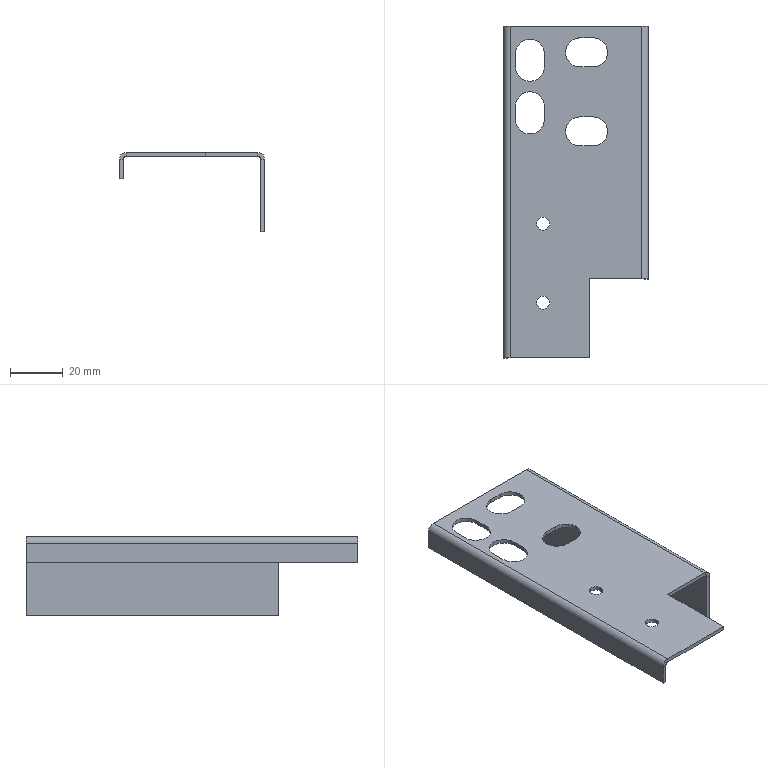Part | 1 solid | 46 faces | box 55 x 126 x 30 mm | volume 13884 mm3 | plane 28 | cylinder 18 | commonest cylinder face diameters 11 x10 5 x6 2 x2
STEP:
#1=CARTESIAN_POINT('',(12.,53.,-1.5));
#2=VERTEX_POINT('',#1);
#3=CARTESIAN_POINT('',(6.5,58.5,-1.5));
#4=VERTEX_POINT('',#3);
#5=CARTESIAN_POINT('',(6.5,53.,-1.5));
#6=DIRECTION('',(0.,0.,1.));
#7=DIRECTION('',(1.,0.,0.));
#8=AXIS2_PLACEMENT_3D('',#5,#6,#7);
#9=CIRCLE('',#8,5.5);
#10=EDGE_CURVE('',#2,#4,#9,.T.);
#11=ORIENTED_EDGE('',*,*,#10,.F.);
#12=CARTESIAN_POINT('',(12.,53.,0.));
#13=VERTEX_POINT('',#12);
#14=CARTESIAN_POINT('',(12.,53.,-10.));
#15=DIRECTION('',(0.,0.,1.));
#16=VECTOR('',#15,1000.);
#17=LINE('',#14,#16);
#18=EDGE_CURVE('',#2,#13,#17,.T.);
#19=ORIENTED_EDGE('',*,*,#18,.T.);
#20=CARTESIAN_POINT('',(6.5,58.5,0.));
#21=VERTEX_POINT('',#20);
#22=CARTESIAN_POINT('',(6.5,53.,0.));
#23=DIRECTION('',(0.,0.,1.));
#24=DIRECTION('',(1.,0.,0.));
#25=AXIS2_PLACEMENT_3D('',#22,#23,#24);
#26=CIRCLE('',#25,5.5);
#27=EDGE_CURVE('',#13,#21,#26,.T.);
#28=ORIENTED_EDGE('',*,*,#27,.T.);
#29=CARTESIAN_POINT('',(6.5,58.5,-10.));
#30=DIRECTION('',(0.,0.,1.));
#31=VECTOR('',#30,1000.);
#32=LINE('',#29,#31);
#33=EDGE_CURVE('',#4,#21,#32,.T.);
#34=ORIENTED_EDGE('',*,*,#33,.F.);
#35=EDGE_LOOP('',(#11,#19,#28,#34));
#36=FACE_OUTER_BOUND('',#35,.T.);
#37=CARTESIAN_POINT('',(6.5,53.,-10.));
#38=DIRECTION('',(0.,0.,1.));
#39=DIRECTION('',(1.,0.,0.));
#40=AXIS2_PLACEMENT_3D('',#37,#38,#39);
#41=CYLINDRICAL_SURFACE('',#40,5.5);
#42=ADVANCED_FACE('',(#36),#41,.F.);
#43=CARTESIAN_POINT('',(12.,23.,-1.5));
#44=VERTEX_POINT('',#43);
#45=CARTESIAN_POINT('',(6.5,28.5,-1.5));
#46=VERTEX_POINT('',#45);
#47=CARTESIAN_POINT('',(6.5,23.,-1.5));
#48=DIRECTION('',(0.,0.,1.));
#49=DIRECTION('',(1.,0.,0.));
#50=AXIS2_PLACEMENT_3D('',#47,#48,#49);
#51=CIRCLE('',#50,5.5);
#52=EDGE_CURVE('',#44,#46,#51,.T.);
#53=ORIENTED_EDGE('',*,*,#52,.F.);
#54=CARTESIAN_POINT('',(12.,23.,0.));
#55=VERTEX_POINT('',#54);
#56=CARTESIAN_POINT('',(12.,23.,-10.));
#57=DIRECTION('',(0.,0.,1.));
#58=VECTOR('',#57,1000.);
#59=LINE('',#56,#58);
#60=EDGE_CURVE('',#44,#55,#59,.T.);
#61=ORIENTED_EDGE('',*,*,#60,.T.);
#62=CARTESIAN_POINT('',(6.5,28.5,0.));
#63=VERTEX_POINT('',#62);
#64=CARTESIAN_POINT('',(6.5,23.,0.));
#65=DIRECTION('',(0.,0.,1.));
#66=DIRECTION('',(1.,0.,0.));
#67=AXIS2_PLACEMENT_3D('',#64,#65,#66);
#68=CIRCLE('',#67,5.5);
#69=EDGE_CURVE('',#55,#63,#68,.T.);
#70=ORIENTED_EDGE('',*,*,#69,.T.);
#71=CARTESIAN_POINT('',(6.5,28.5,-10.));
#72=DIRECTION('',(0.,0.,1.));
#73=VECTOR('',#72,1000.);
#74=LINE('',#71,#73);
#75=EDGE_CURVE('',#46,#63,#74,.T.);
#76=ORIENTED_EDGE('',*,*,#75,.F.);
#77=EDGE_LOOP('',(#53,#61,#70,#76));
#78=FACE_OUTER_BOUND('',#77,.T.);
#79=CARTESIAN_POINT('',(6.5,23.,-10.));
#80=DIRECTION('',(0.,0.,1.));
#81=DIRECTION('',(1.,0.,0.));
#82=AXIS2_PLACEMENT_3D('',#79,#80,#81);
#83=CYLINDRICAL_SURFACE('',#82,5.5);
#84=ADVANCED_FACE('',(#78),#83,.F.);
#85=CARTESIAN_POINT('',(-15.,-42.,-1.5));
#86=VERTEX_POINT('',#85);
#87=CARTESIAN_POINT('',(-10.,-42.,-1.5));
#88=VERTEX_POINT('',#87);
#89=CARTESIAN_POINT('',(-12.5,-42.,-1.5));
#90=DIRECTION('',(0.,0.,1.));
#91=DIRECTION('',(1.,0.,0.));
#92=AXIS2_PLACEMENT_3D('',#89,#90,#91);
#93=CIRCLE('',#92,2.5);
#94=EDGE_CURVE('',#86,#88,#93,.T.);
#95=ORIENTED_EDGE('',*,*,#94,.F.);
#96=CARTESIAN_POINT('',(-15.,-42.,0.));
#97=VERTEX_POINT('',#96);
#98=CARTESIAN_POINT('',(-15.,-42.,-10.));
#99=DIRECTION('',(0.,0.,1.));
#100=VECTOR('',#99,1000.);
#101=LINE('',#98,#100);
#102=EDGE_CURVE('',#86,#97,#101,.T.);
#103=ORIENTED_EDGE('',*,*,#102,.T.);
#104=CARTESIAN_POINT('',(-10.,-42.,0.));
#105=VERTEX_POINT('',#104);
#106=CARTESIAN_POINT('',(-12.5,-42.,0.));
#107=DIRECTION('',(0.,0.,1.));
#108=DIRECTION('',(1.,0.,0.));
#109=AXIS2_PLACEMENT_3D('',#106,#107,#108);
#110=CIRCLE('',#109,2.5);
#111=EDGE_CURVE('',#97,#105,#110,.T.);
#112=ORIENTED_EDGE('',*,*,#111,.T.);
#113=CARTESIAN_POINT('',(-10.,-42.,-10.));
#114=DIRECTION('',(0.,0.,1.));
#115=VECTOR('',#114,1000.);
#116=LINE('',#113,#115);
#117=EDGE_CURVE('',#88,#105,#116,.T.);
#118=ORIENTED_EDGE('',*,*,#117,.F.);
#119=EDGE_LOOP('',(#95,#103,#112,#118));
#120=FACE_OUTER_BOUND('',#119,.T.);
#121=CARTESIAN_POINT('',(-12.5,-42.,-10.));
#122=DIRECTION('',(0.,0.,1.));
#123=DIRECTION('',(1.,0.,0.));
#124=AXIS2_PLACEMENT_3D('',#121,#122,#123);
#125=CYLINDRICAL_SURFACE('',#124,2.5);
#126=ADVANCED_FACE('',(#120),#125,.F.);
#127=CARTESIAN_POINT('',(-15.,-12.,-1.5));
#128=VERTEX_POINT('',#127);
#129=CARTESIAN_POINT('',(-10.,-12.,-1.5));
#130=VERTEX_POINT('',#129);
#131=CARTESIAN_POINT('',(-12.5,-12.,-1.5));
#132=DIRECTION('',(0.,0.,1.));
#133=DIRECTION('',(1.,0.,0.));
#134=AXIS2_PLACEMENT_3D('',#131,#132,#133);
#135=CIRCLE('',#134,2.5);
#136=EDGE_CURVE('',#128,#130,#135,.T.);
#137=ORIENTED_EDGE('',*,*,#136,.F.);
#138=CARTESIAN_POINT('',(-15.,-12.,0.));
#139=VERTEX_POINT('',#138);
#140=CARTESIAN_POINT('',(-15.,-12.,-10.));
#141=DIRECTION('',(0.,0.,1.));
#142=VECTOR('',#141,1000.);
#143=LINE('',#140,#142);
#144=EDGE_CURVE('',#128,#139,#143,.T.);
#145=ORIENTED_EDGE('',*,*,#144,.T.);
#146=CARTESIAN_POINT('',(-10.,-12.,0.));
#147=VERTEX_POINT('',#146);
#148=CARTESIAN_POINT('',(-12.5,-12.,0.));
#149=DIRECTION('',(0.,0.,1.));
#150=DIRECTION('',(1.,0.,0.));
#151=AXIS2_PLACEMENT_3D('',#148,#149,#150);
#152=CIRCLE('',#151,2.5);
#153=EDGE_CURVE('',#139,#147,#152,.T.);
#154=ORIENTED_EDGE('',*,*,#153,.T.);
#155=CARTESIAN_POINT('',(-10.,-12.,-10.));
#156=DIRECTION('',(0.,0.,1.));
#157=VECTOR('',#156,1000.);
#158=LINE('',#155,#157);
#159=EDGE_CURVE('',#130,#147,#158,.T.);
#160=ORIENTED_EDGE('',*,*,#159,.F.);
#161=EDGE_LOOP('',(#137,#145,#154,#160));
#162=FACE_OUTER_BOUND('',#161,.T.);
#163=CARTESIAN_POINT('',(-12.5,-12.,-10.));
#164=DIRECTION('',(0.,0.,1.));
#165=DIRECTION('',(1.,0.,0.));
#166=AXIS2_PLACEMENT_3D('',#163,#164,#165);
#167=CYLINDRICAL_SURFACE('',#166,2.5);
#168=ADVANCED_FACE('',(#162),#167,.F.);
#169=CARTESIAN_POINT('',(27.5,-33.,-30.));
#170=VERTEX_POINT('',#169);
#171=CARTESIAN_POINT('',(27.5,-33.,-2.5));
#172=VERTEX_POINT('',#171);
#173=CARTESIAN_POINT('',(27.5,-33.,-30.));
#174=DIRECTION('',(0.,0.,1.));
#175=VECTOR('',#174,1000.);
#176=LINE('',#173,#175);
#177=EDGE_CURVE('',#170,#172,#176,.T.);
#178=ORIENTED_EDGE('',*,*,#177,.T.);
#179=CARTESIAN_POINT('',(26.,-33.,-2.5));
#180=VERTEX_POINT('',#179);
#181=CARTESIAN_POINT('',(27.5,-33.,-2.5));
#182=DIRECTION('',(-1.,0.,0.));
#183=VECTOR('',#182,1000.);
#184=LINE('',#181,#183);
#185=EDGE_CURVE('',#172,#180,#184,.T.);
#186=ORIENTED_EDGE('',*,*,#185,.T.);
#187=CARTESIAN_POINT('',(26.,-33.,-30.));
#188=VERTEX_POINT('',#187);
#189=CARTESIAN_POINT('',(26.,-33.,0.));
#190=DIRECTION('',(0.,0.,1.));
#191=VECTOR('',#190,1000.);
#192=LINE('',#189,#191);
#193=EDGE_CURVE('',#188,#180,#192,.T.);
#194=ORIENTED_EDGE('',*,*,#193,.F.);
#195=CARTESIAN_POINT('',(27.5,-33.,-30.));
#196=DIRECTION('',(-1.,0.,0.));
#197=VECTOR('',#196,1000.);
#198=LINE('',#195,#197);
#199=EDGE_CURVE('',#170,#188,#198,.T.);
#200=ORIENTED_EDGE('',*,*,#199,.F.);
#201=EDGE_LOOP('',(#178,#186,#194,#200));
#202=FACE_OUTER_BOUND('',#201,.T.);
#203=CARTESIAN_POINT('',(27.5,-33.,-30.));
#204=DIRECTION('',(0.,1.,0.));
#205=DIRECTION('',(0.,0.,1.));
#206=AXIS2_PLACEMENT_3D('',#203,#204,#205);
#207=PLANE('',#206);
#208=ADVANCED_FACE('',(#202),#207,.F.);
#209=CARTESIAN_POINT('',(25.,-33.,-1.5));
#210=VERTEX_POINT('',#209);
#211=CARTESIAN_POINT('',(5.,-33.,-1.5));
#212=VERTEX_POINT('',#211);
#213=CARTESIAN_POINT('',(0.,-33.,-1.5));
#214=DIRECTION('',(-1.,0.,0.));
#215=VECTOR('',#214,1000.);
#216=LINE('',#213,#215);
#217=EDGE_CURVE('',#210,#212,#216,.T.);
#218=ORIENTED_EDGE('',*,*,#217,.F.);
#219=CARTESIAN_POINT('',(25.,-33.,0.));
#220=VERTEX_POINT('',#219);
#221=CARTESIAN_POINT('',(25.,-33.,-1.5));
#222=DIRECTION('',(0.,0.,1.));
#223=VECTOR('',#222,1000.);
#224=LINE('',#221,#223);
#225=EDGE_CURVE('',#210,#220,#224,.T.);
#226=ORIENTED_EDGE('',*,*,#225,.T.);
#227=CARTESIAN_POINT('',(5.,-33.,0.));
#228=VERTEX_POINT('',#227);
#229=CARTESIAN_POINT('',(0.,-33.,0.));
#230=DIRECTION('',(-1.,0.,0.));
#231=VECTOR('',#230,1000.);
#232=LINE('',#229,#231);
#233=EDGE_CURVE('',#220,#228,#232,.T.);
#234=ORIENTED_EDGE('',*,*,#233,.T.);
#235=CARTESIAN_POINT('',(5.,-33.,-30.));
#236=DIRECTION('',(0.,0.,1.));
#237=VECTOR('',#236,1000.);
#238=LINE('',#235,#237);
#239=EDGE_CURVE('',#212,#228,#238,.T.);
#240=ORIENTED_EDGE('',*,*,#239,.F.);
#241=EDGE_LOOP('',(#218,#226,#234,#240));
#242=FACE_OUTER_BOUND('',#241,.T.);
#243=CARTESIAN_POINT('',(27.5,-33.,-30.));
#244=DIRECTION('',(0.,1.,0.));
#245=DIRECTION('',(0.,0.,1.));
#246=AXIS2_PLACEMENT_3D('',#243,#244,#245);
#247=PLANE('',#246);
#248=ADVANCED_FACE('',(#242),#247,.F.);
#249=CARTESIAN_POINT('',(-12.,47.5,-1.5));
#250=VERTEX_POINT('',#249);
#251=CARTESIAN_POINT('',(-12.,52.5,-1.5));
#252=VERTEX_POINT('',#251);
#253=CARTESIAN_POINT('',(-12.,0.,-1.5));
#254=DIRECTION('',(0.,1.,0.));
#255=VECTOR('',#254,1000.);
#256=LINE('',#253,#255);
#257=EDGE_CURVE('',#250,#252,#256,.T.);
#258=ORIENTED_EDGE('',*,*,#257,.T.);
#259=CARTESIAN_POINT('',(-23.,52.5,-1.5));
#260=VERTEX_POINT('',#259);
#261=CARTESIAN_POINT('',(-17.5,52.5,-1.5));
#262=DIRECTION('',(0.,0.,1.));
#263=DIRECTION('',(1.,0.,0.));
#264=AXIS2_PLACEMENT_3D('',#261,#262,#263);
#265=CIRCLE('',#264,5.5);
#266=EDGE_CURVE('',#252,#260,#265,.T.);
#267=ORIENTED_EDGE('',*,*,#266,.T.);
#268=CARTESIAN_POINT('',(-23.,47.5,-1.5));
#269=VERTEX_POINT('',#268);
#270=CARTESIAN_POINT('',(-23.,0.,-1.5));
#271=DIRECTION('',(0.,-1.,0.));
#272=VECTOR('',#271,1000.);
#273=LINE('',#270,#272);
#274=EDGE_CURVE('',#260,#269,#273,.T.);
#275=ORIENTED_EDGE('',*,*,#274,.T.);
#276=CARTESIAN_POINT('',(-17.5,47.5,-1.5));
#277=DIRECTION('',(0.,0.,1.));
#278=DIRECTION('',(1.,0.,0.));
#279=AXIS2_PLACEMENT_3D('',#276,#277,#278);
#280=CIRCLE('',#279,5.5);
#281=EDGE_CURVE('',#269,#250,#280,.T.);
#282=ORIENTED_EDGE('',*,*,#281,.T.);
#283=EDGE_LOOP('',(#258,#267,#275,#282));
#284=FACE_BOUND('',#283,.T.);
#285=CARTESIAN_POINT('',(-12.,27.5,-1.5));
#286=VERTEX_POINT('',#285);
#287=CARTESIAN_POINT('',(-12.,32.5,-1.5));
#288=VERTEX_POINT('',#287);
#289=CARTESIAN_POINT('',(-12.,0.,-1.5));
#290=DIRECTION('',(0.,1.,0.));
#291=VECTOR('',#290,1000.);
#292=LINE('',#289,#291);
#293=EDGE_CURVE('',#286,#288,#292,.T.);
#294=ORIENTED_EDGE('',*,*,#293,.T.);
#295=CARTESIAN_POINT('',(-23.,32.5,-1.5));
#296=VERTEX_POINT('',#295);
#297=CARTESIAN_POINT('',(-17.5,32.5,-1.5));
#298=DIRECTION('',(0.,0.,1.));
#299=DIRECTION('',(1.,0.,0.));
#300=AXIS2_PLACEMENT_3D('',#297,#298,#299);
#301=CIRCLE('',#300,5.5);
#302=EDGE_CURVE('',#288,#296,#301,.T.);
#303=ORIENTED_EDGE('',*,*,#302,.T.);
#304=CARTESIAN_POINT('',(-23.,27.5,-1.5));
#305=VERTEX_POINT('',#304);
#306=CARTESIAN_POINT('',(-23.,0.,-1.5));
#307=DIRECTION('',(0.,-1.,0.));
#308=VECTOR('',#307,1000.);
#309=LINE('',#306,#308);
#310=EDGE_CURVE('',#296,#305,#309,.T.);
#311=ORIENTED_EDGE('',*,*,#310,.T.);
#312=CARTESIAN_POINT('',(-17.5,27.5,-1.5));
#313=DIRECTION('',(0.,0.,1.));
#314=DIRECTION('',(1.,0.,0.));
#315=AXIS2_PLACEMENT_3D('',#312,#313,#314);
#316=CIRCLE('',#315,5.5);
#317=EDGE_CURVE('',#305,#286,#316,.T.);
#318=ORIENTED_EDGE('',*,*,#317,.T.);
#319=EDGE_LOOP('',(#294,#303,#311,#318));
#320=FACE_BOUND('',#319,.T.);
#321=CARTESIAN_POINT('',(1.5,58.5,-1.5));
#322=VERTEX_POINT('',#321);
#323=CARTESIAN_POINT('',(0.,58.5,-1.5));
#324=DIRECTION('',(-1.,0.,0.));
#325=VECTOR('',#324,1000.);
#326=LINE('',#323,#325);
#327=EDGE_CURVE('',#4,#322,#326,.T.);
#328=ORIENTED_EDGE('',*,*,#327,.T.);
#329=CARTESIAN_POINT('',(1.5,47.5,-1.5));
#330=VERTEX_POINT('',#329);
#331=CARTESIAN_POINT('',(1.5,53.,-1.5));
#332=DIRECTION('',(0.,0.,1.));
#333=DIRECTION('',(1.,0.,0.));
#334=AXIS2_PLACEMENT_3D('',#331,#332,#333);
#335=CIRCLE('',#334,5.5);
#336=EDGE_CURVE('',#322,#330,#335,.T.);
#337=ORIENTED_EDGE('',*,*,#336,.T.);
#338=CARTESIAN_POINT('',(6.5,47.5,-1.5));
#339=VERTEX_POINT('',#338);
#340=CARTESIAN_POINT('',(0.,47.5,-1.5));
#341=DIRECTION('',(1.,0.,0.));
#342=VECTOR('',#341,1000.);
#343=LINE('',#340,#342);
#344=EDGE_CURVE('',#330,#339,#343,.T.);
#345=ORIENTED_EDGE('',*,*,#344,.T.);
#346=CARTESIAN_POINT('',(6.5,53.,-1.5));
#347=DIRECTION('',(0.,0.,1.));
#348=DIRECTION('',(1.,0.,0.));
#349=AXIS2_PLACEMENT_3D('',#346,#347,#348);
#350=CIRCLE('',#349,5.5);
#351=EDGE_CURVE('',#339,#2,#350,.T.);
#352=ORIENTED_EDGE('',*,*,#351,.T.);
#353=ORIENTED_EDGE('',*,*,#10,.T.);
#354=EDGE_LOOP('',(#328,#337,#345,#352,#353));
#355=FACE_BOUND('',#354,.T.);
#356=CARTESIAN_POINT('',(1.5,28.5,-1.5));
#357=VERTEX_POINT('',#356);
#358=CARTESIAN_POINT('',(0.,28.5,-1.5));
#359=DIRECTION('',(-1.,0.,0.));
#360=VECTOR('',#359,1000.);
#361=LINE('',#358,#360);
#362=EDGE_CURVE('',#46,#357,#361,.T.);
#363=ORIENTED_EDGE('',*,*,#362,.T.);
#364=CARTESIAN_POINT('',(1.5,17.5,-1.5));
#365=VERTEX_POINT('',#364);
#366=CARTESIAN_POINT('',(1.5,23.,-1.5));
#367=DIRECTION('',(0.,0.,1.));
#368=DIRECTION('',(1.,0.,0.));
#369=AXIS2_PLACEMENT_3D('',#366,#367,#368);
#370=CIRCLE('',#369,5.5);
#371=EDGE_CURVE('',#357,#365,#370,.T.);
#372=ORIENTED_EDGE('',*,*,#371,.T.);
#373=CARTESIAN_POINT('',(6.5,17.5,-1.5));
#374=VERTEX_POINT('',#373);
#375=CARTESIAN_POINT('',(0.,17.5,-1.5));
#376=DIRECTION('',(1.,0.,0.));
#377=VECTOR('',#376,1000.);
#378=LINE('',#375,#377);
#379=EDGE_CURVE('',#365,#374,#378,.T.);
#380=ORIENTED_EDGE('',*,*,#379,.T.);
#381=CARTESIAN_POINT('',(6.5,23.,-1.5));
#382=DIRECTION('',(0.,0.,1.));
#383=DIRECTION('',(1.,0.,0.));
#384=AXIS2_PLACEMENT_3D('',#381,#382,#383);
#385=CIRCLE('',#384,5.5);
#386=EDGE_CURVE('',#374,#44,#385,.T.);
#387=ORIENTED_EDGE('',*,*,#386,.T.);
#388=ORIENTED_EDGE('',*,*,#52,.T.);
#389=EDGE_LOOP('',(#363,#372,#380,#387,#388));
#390=FACE_BOUND('',#389,.T.);
#391=CARTESIAN_POINT('',(-12.5,-42.,-1.5));
#392=DIRECTION('',(0.,0.,1.));
#393=DIRECTION('',(1.,0.,0.));
#394=AXIS2_PLACEMENT_3D('',#391,#392,#393);
#395=CIRCLE('',#394,2.5);
#396=EDGE_CURVE('',#88,#86,#395,.T.);
#397=ORIENTED_EDGE('',*,*,#396,.T.);
#398=ORIENTED_EDGE('',*,*,#94,.T.);
#399=EDGE_LOOP('',(#397,#398));
#400=FACE_BOUND('',#399,.T.);
#401=CARTESIAN_POINT('',(-12.5,-12.,-1.5));
#402=DIRECTION('',(0.,0.,1.));
#403=DIRECTION('',(1.,0.,0.));
#404=AXIS2_PLACEMENT_3D('',#401,#402,#403);
#405=CIRCLE('',#404,2.5);
#406=EDGE_CURVE('',#130,#128,#405,.T.);
#407=ORIENTED_EDGE('',*,*,#406,.T.);
#408=ORIENTED_EDGE('',*,*,#136,.T.);
#409=EDGE_LOOP('',(#407,#408));
#410=FACE_BOUND('',#409,.T.);
#411=ORIENTED_EDGE('',*,*,#217,.T.);
#412=CARTESIAN_POINT('',(5.,-63.,-1.5));
#413=VERTEX_POINT('',#412);
#414=CARTESIAN_POINT('',(5.,0.,-1.5));
#415=DIRECTION('',(0.,-1.,0.));
#416=VECTOR('',#415,1000.);
#417=LINE('',#414,#416);
#418=EDGE_CURVE('',#212,#413,#417,.T.);
#419=ORIENTED_EDGE('',*,*,#418,.T.);
#420=CARTESIAN_POINT('',(-25.,-63.,-1.5));
#421=VERTEX_POINT('',#420);
#422=CARTESIAN_POINT('',(-27.5,-63.,-1.5));
#423=DIRECTION('',(1.,0.,0.));
#424=VECTOR('',#423,1000.);
#425=LINE('',#422,#424);
#426=EDGE_CURVE('',#421,#413,#425,.T.);
#427=ORIENTED_EDGE('',*,*,#426,.F.);
#428=CARTESIAN_POINT('',(-25.,63.,-1.5));
#429=VERTEX_POINT('',#428);
#430=CARTESIAN_POINT('',(-25.,63.,-1.5));
#431=DIRECTION('',(0.,-1.,0.));
#432=VECTOR('',#431,1000.);
#433=LINE('',#430,#432);
#434=EDGE_CURVE('',#429,#421,#433,.T.);
#435=ORIENTED_EDGE('',*,*,#434,.F.);
#436=CARTESIAN_POINT('',(25.,63.,-1.5));
#437=VERTEX_POINT('',#436);
#438=CARTESIAN_POINT('',(-27.5,63.,-1.5));
#439=DIRECTION('',(-1.,0.,0.));
#440=VECTOR('',#439,1000.);
#441=LINE('',#438,#440);
#442=EDGE_CURVE('',#437,#429,#441,.T.);
#443=ORIENTED_EDGE('',*,*,#442,.F.);
#444=CARTESIAN_POINT('',(25.,-63.,-1.5));
#445=DIRECTION('',(0.,1.,0.));
#446=VECTOR('',#445,1000.);
#447=LINE('',#444,#446);
#448=EDGE_CURVE('',#210,#437,#447,.T.);
#449=ORIENTED_EDGE('',*,*,#448,.F.);
#450=EDGE_LOOP('',(#411,#419,#427,#435,#443,#449));
#451=FACE_OUTER_BOUND('',#450,.T.);
#452=CARTESIAN_POINT('',(0.,0.,-1.5));
#453=DIRECTION('',(0.,0.,1.));
#454=DIRECTION('',(1.,0.,0.));
#455=AXIS2_PLACEMENT_3D('',#452,#453,#454);
#456=PLANE('',#455);
#457=ADVANCED_FACE('',(#284,#320,#355,#390,#400,#410,#451),#456,.F.);
#458=CARTESIAN_POINT('',(-12.,52.5,0.));
#459=VERTEX_POINT('',#458);
#460=CARTESIAN_POINT('',(-23.,52.5,0.));
#461=VERTEX_POINT('',#460);
#462=CARTESIAN_POINT('',(-17.5,52.5,0.));
#463=DIRECTION('',(0.,0.,1.));
#464=DIRECTION('',(1.,0.,0.));
#465=AXIS2_PLACEMENT_3D('',#462,#463,#464);
#466=CIRCLE('',#465,5.5);
#467=EDGE_CURVE('',#459,#461,#466,.T.);
#468=ORIENTED_EDGE('',*,*,#467,.F.);
#469=CARTESIAN_POINT('',(-12.,47.5,0.));
#470=VERTEX_POINT('',#469);
#471=CARTESIAN_POINT('',(-12.,52.5,0.));
#472=DIRECTION('',(0.,1.,0.));
#473=VECTOR('',#472,1000.);
#474=LINE('',#471,#473);
#475=EDGE_CURVE('',#470,#459,#474,.T.);
#476=ORIENTED_EDGE('',*,*,#475,.F.);
#477=CARTESIAN_POINT('',(-23.,47.5,0.));
#478=VERTEX_POINT('',#477);
#479=CARTESIAN_POINT('',(-17.5,47.5,0.));
#480=DIRECTION('',(0.,0.,1.));
#481=DIRECTION('',(1.,0.,0.));
#482=AXIS2_PLACEMENT_3D('',#479,#480,#481);
#483=CIRCLE('',#482,5.5);
#484=EDGE_CURVE('',#478,#470,#483,.T.);
#485=ORIENTED_EDGE('',*,*,#484,.F.);
#486=CARTESIAN_POINT('',(-23.,52.5,0.));
#487=DIRECTION('',(0.,-1.,0.));
#488=VECTOR('',#487,1000.);
#489=LINE('',#486,#488);
#490=EDGE_CURVE('',#461,#478,#489,.T.);
#491=ORIENTED_EDGE('',*,*,#490,.F.);
#492=EDGE_LOOP('',(#468,#476,#485,#491));
#493=FACE_BOUND('',#492,.T.);
#494=CARTESIAN_POINT('',(-12.,32.5,0.));
#495=VERTEX_POINT('',#494);
#496=CARTESIAN_POINT('',(-23.,32.5,0.));
#497=VERTEX_POINT('',#496);
#498=CARTESIAN_POINT('',(-17.5,32.5,0.));
#499=DIRECTION('',(0.,0.,1.));
#500=DIRECTION('',(1.,0.,0.));
#501=AXIS2_PLACEMENT_3D('',#498,#499,#500);
#502=CIRCLE('',#501,5.5);
#503=EDGE_CURVE('',#495,#497,#502,.T.);
#504=ORIENTED_EDGE('',*,*,#503,.F.);
#505=CARTESIAN_POINT('',(-12.,27.5,0.));
#506=VERTEX_POINT('',#505);
#507=CARTESIAN_POINT('',(-12.,32.5,0.));
#508=DIRECTION('',(0.,1.,0.));
#509=VECTOR('',#508,1000.);
#510=LINE('',#507,#509);
#511=EDGE_CURVE('',#506,#495,#510,.T.);
#512=ORIENTED_EDGE('',*,*,#511,.F.);
#513=CARTESIAN_POINT('',(-23.,27.5,0.));
#514=VERTEX_POINT('',#513);
#515=CARTESIAN_POINT('',(-17.5,27.5,0.));
#516=DIRECTION('',(0.,0.,1.));
#517=DIRECTION('',(1.,0.,0.));
#518=AXIS2_PLACEMENT_3D('',#515,#516,#517);
#519=CIRCLE('',#518,5.5);
#520=EDGE_CURVE('',#514,#506,#519,.T.);
#521=ORIENTED_EDGE('',*,*,#520,.F.);
#522=CARTESIAN_POINT('',(-23.,32.5,0.));
#523=DIRECTION('',(0.,-1.,0.));
#524=VECTOR('',#523,1000.);
#525=LINE('',#522,#524);
#526=EDGE_CURVE('',#497,#514,#525,.T.);
#527=ORIENTED_EDGE('',*,*,#526,.F.);
#528=EDGE_LOOP('',(#504,#512,#521,#527));
#529=FACE_BOUND('',#528,.T.);
#530=CARTESIAN_POINT('',(1.5,58.5,0.));
#531=VERTEX_POINT('',#530);
#532=CARTESIAN_POINT('',(1.5,47.5,0.));
#533=VERTEX_POINT('',#532);
#534=CARTESIAN_POINT('',(1.5,53.,0.));
#535=DIRECTION('',(0.,0.,1.));
#536=DIRECTION('',(1.,0.,0.));
#537=AXIS2_PLACEMENT_3D('',#534,#535,#536);
#538=CIRCLE('',#537,5.5);
#539=EDGE_CURVE('',#531,#533,#538,.T.);
#540=ORIENTED_EDGE('',*,*,#539,.F.);
#541=CARTESIAN_POINT('',(1.5,58.5,0.));
#542=DIRECTION('',(-1.,0.,0.));
#543=VECTOR('',#542,1000.);
#544=LINE('',#541,#543);
#545=EDGE_CURVE('',#21,#531,#544,.T.);
#546=ORIENTED_EDGE('',*,*,#545,.F.);
#547=ORIENTED_EDGE('',*,*,#27,.F.);
#548=CARTESIAN_POINT('',(6.5,47.5,0.));
#549=VERTEX_POINT('',#548);
#550=CARTESIAN_POINT('',(6.5,53.,0.));
#551=DIRECTION('',(0.,0.,1.));
#552=DIRECTION('',(1.,0.,0.));
#553=AXIS2_PLACEMENT_3D('',#550,#551,#552);
#554=CIRCLE('',#553,5.5);
#555=EDGE_CURVE('',#549,#13,#554,.T.);
#556=ORIENTED_EDGE('',*,*,#555,.F.);
#557=CARTESIAN_POINT('',(1.5,47.5,0.));
#558=DIRECTION('',(1.,0.,0.));
#559=VECTOR('',#558,1000.);
#560=LINE('',#557,#559);
#561=EDGE_CURVE('',#533,#549,#560,.T.);
#562=ORIENTED_EDGE('',*,*,#561,.F.);
#563=EDGE_LOOP('',(#540,#546,#547,#556,#562));
#564=FACE_BOUND('',#563,.T.);
#565=CARTESIAN_POINT('',(1.5,28.5,0.));
#566=VERTEX_POINT('',#565);
#567=CARTESIAN_POINT('',(1.5,17.5,0.));
#568=VERTEX_POINT('',#567);
#569=CARTESIAN_POINT('',(1.5,23.,0.));
#570=DIRECTION('',(0.,0.,1.));
#571=DIRECTION('',(1.,0.,0.));
#572=AXIS2_PLACEMENT_3D('',#569,#570,#571);
#573=CIRCLE('',#572,5.5);
#574=EDGE_CURVE('',#566,#568,#573,.T.);
#575=ORIENTED_EDGE('',*,*,#574,.F.);
#576=CARTESIAN_POINT('',(1.5,28.5,0.));
#577=DIRECTION('',(-1.,0.,0.));
#578=VECTOR('',#577,1000.);
#579=LINE('',#576,#578);
#580=EDGE_CURVE('',#63,#566,#579,.T.);
#581=ORIENTED_EDGE('',*,*,#580,.F.);
#582=ORIENTED_EDGE('',*,*,#69,.F.);
#583=CARTESIAN_POINT('',(6.5,17.5,0.));
#584=VERTEX_POINT('',#583);
#585=CARTESIAN_POINT('',(6.5,23.,0.));
#586=DIRECTION('',(0.,0.,1.));
#587=DIRECTION('',(1.,0.,0.));
#588=AXIS2_PLACEMENT_3D('',#585,#586,#587);
#589=CIRCLE('',#588,5.5);
#590=EDGE_CURVE('',#584,#55,#589,.T.);
#591=ORIENTED_EDGE('',*,*,#590,.F.);
#592=CARTESIAN_POINT('',(1.5,17.5,0.));
#593=DIRECTION('',(1.,0.,0.));
#594=VECTOR('',#593,1000.);
#595=LINE('',#592,#594);
#596=EDGE_CURVE('',#568,#584,#595,.T.);
#597=ORIENTED_EDGE('',*,*,#596,.F.);
#598=EDGE_LOOP('',(#575,#581,#582,#591,#597));
#599=FACE_BOUND('',#598,.T.);
#600=CARTESIAN_POINT('',(-12.5,-42.,0.));
#601=DIRECTION('',(0.,0.,1.));
#602=DIRECTION('',(1.,0.,0.));
#603=AXIS2_PLACEMENT_3D('',#600,#601,#602);
#604=CIRCLE('',#603,2.5);
#605=EDGE_CURVE('',#105,#97,#604,.T.);
#606=ORIENTED_EDGE('',*,*,#605,.F.);
#607=ORIENTED_EDGE('',*,*,#111,.F.);
#608=EDGE_LOOP('',(#606,#607));
#609=FACE_BOUND('',#608,.T.);
#610=CARTESIAN_POINT('',(-12.5,-12.,0.));
#611=DIRECTION('',(0.,0.,1.));
#612=DIRECTION('',(1.,0.,0.));
#613=AXIS2_PLACEMENT_3D('',#610,#611,#612);
#614=CIRCLE('',#613,2.5);
#615=EDGE_CURVE('',#147,#139,#614,.T.);
#616=ORIENTED_EDGE('',*,*,#615,.F.);
#617=ORIENTED_EDGE('',*,*,#153,.F.);
#618=EDGE_LOOP('',(#616,#617));
#619=FACE_BOUND('',#618,.T.);
#620=CARTESIAN_POINT('',(5.,-63.,0.));
#621=VERTEX_POINT('',#620);
#622=CARTESIAN_POINT('',(5.,0.,0.));
#623=DIRECTION('',(0.,-1.,0.));
#624=VECTOR('',#623,1000.);
#625=LINE('',#622,#624);
#626=EDGE_CURVE('',#228,#621,#625,.T.);
#627=ORIENTED_EDGE('',*,*,#626,.F.);
#628=ORIENTED_EDGE('',*,*,#233,.F.);
#629=CARTESIAN_POINT('',(25.,63.,0.));
#630=VERTEX_POINT('',#629);
#631=CARTESIAN_POINT('',(25.,-63.,0.));
#632=DIRECTION('',(0.,1.,0.));
#633=VECTOR('',#632,1000.);
#634=LINE('',#631,#633);
#635=EDGE_CURVE('',#220,#630,#634,.T.);
#636=ORIENTED_EDGE('',*,*,#635,.T.);
#637=CARTESIAN_POINT('',(-25.,63.,0.));
#638=VERTEX_POINT('',#637);
#639=CARTESIAN_POINT('',(-27.5,63.,0.));
#640=DIRECTION('',(-1.,0.,0.));
#641=VECTOR('',#640,1000.);
#642=LINE('',#639,#641);
#643=EDGE_CURVE('',#630,#638,#642,.T.);
#644=ORIENTED_EDGE('',*,*,#643,.T.);
#645=CARTESIAN_POINT('',(-25.,-63.,0.));
#646=VERTEX_POINT('',#645);
#647=CARTESIAN_POINT('',(-25.,63.,0.));
#648=DIRECTION('',(0.,-1.,0.));
#649=VECTOR('',#648,1000.);
#650=LINE('',#647,#649);
#651=EDGE_CURVE('',#638,#646,#650,.T.);
#652=ORIENTED_EDGE('',*,*,#651,.T.);
#653=CARTESIAN_POINT('',(-27.5,-63.,0.));
#654=DIRECTION('',(1.,0.,0.));
#655=VECTOR('',#654,1000.);
#656=LINE('',#653,#655);
#657=EDGE_CURVE('',#646,#621,#656,.T.);
#658=ORIENTED_EDGE('',*,*,#657,.T.);
#659=EDGE_LOOP('',(#627,#628,#636,#644,#652,#658));
#660=FACE_OUTER_BOUND('',#659,.T.);
#661=CARTESIAN_POINT('',(0.,0.,0.));
#662=DIRECTION('',(0.,0.,1.));
#663=DIRECTION('',(1.,0.,0.));
#664=AXIS2_PLACEMENT_3D('',#661,#662,#663);
#665=PLANE('',#664);
#666=ADVANCED_FACE('',(#493,#529,#564,#599,#609,#619,#660),#665,.T.);
#667=ORIENTED_EDGE('',*,*,#442,.T.);
#668=CARTESIAN_POINT('',(-25.,63.,-1.5));
#669=DIRECTION('',(0.,0.,1.));
#670=VECTOR('',#669,1000.);
#671=LINE('',#668,#670);
#672=EDGE_CURVE('',#429,#638,#671,.T.);
#673=ORIENTED_EDGE('',*,*,#672,.T.);
#674=ORIENTED_EDGE('',*,*,#643,.F.);
#675=CARTESIAN_POINT('',(25.,63.,-1.5));
#676=DIRECTION('',(0.,0.,1.));
#677=VECTOR('',#676,1000.);
#678=LINE('',#675,#677);
#679=EDGE_CURVE('',#437,#630,#678,.T.);
#680=ORIENTED_EDGE('',*,*,#679,.F.);
#681=EDGE_LOOP('',(#667,#673,#674,#680));
#682=FACE_OUTER_BOUND('',#681,.T.);
#683=CARTESIAN_POINT('',(-27.5,63.,-1.5));
#684=DIRECTION('',(0.,1.,0.));
#685=DIRECTION('',(0.,0.,1.));
#686=AXIS2_PLACEMENT_3D('',#683,#684,#685);
#687=PLANE('',#686);
#688=ADVANCED_FACE('',(#682),#687,.T.);
#689=CARTESIAN_POINT('',(5.,-63.,-30.));
#690=DIRECTION('',(0.,0.,1.));
#691=VECTOR('',#690,1000.);
#692=LINE('',#689,#691);
#693=EDGE_CURVE('',#413,#621,#692,.T.);
#694=ORIENTED_EDGE('',*,*,#693,.T.);
#695=ORIENTED_EDGE('',*,*,#657,.F.);
#696=CARTESIAN_POINT('',(-25.,-63.,-1.5));
#697=DIRECTION('',(0.,0.,1.));
#698=VECTOR('',#697,1000.);
#699=LINE('',#696,#698);
#700=EDGE_CURVE('',#421,#646,#699,.T.);
#701=ORIENTED_EDGE('',*,*,#700,.F.);
#702=ORIENTED_EDGE('',*,*,#426,.T.);
#703=EDGE_LOOP('',(#694,#695,#701,#702));
#704=FACE_OUTER_BOUND('',#703,.T.);
#705=CARTESIAN_POINT('',(-27.5,-63.,-1.5));
#706=DIRECTION('',(0.,-1.,0.));
#707=DIRECTION('',(0.,0.,-1.));
#708=AXIS2_PLACEMENT_3D('',#705,#706,#707);
#709=PLANE('',#708);
#710=ADVANCED_FACE('',(#704),#709,.T.);
#711=CARTESIAN_POINT('',(26.,63.,-2.5));
#712=VERTEX_POINT('',#711);
#713=CARTESIAN_POINT('',(27.5,63.,-2.5));
#714=VERTEX_POINT('',#713);
#715=CARTESIAN_POINT('',(27.5,63.,-2.5));
#716=DIRECTION('',(1.,0.,0.));
#717=VECTOR('',#716,1000.);
#718=LINE('',#715,#717);
#719=EDGE_CURVE('',#712,#714,#718,.T.);
#720=ORIENTED_EDGE('',*,*,#719,.F.);
#721=CARTESIAN_POINT('',(25.,63.,-2.5));
#722=DIRECTION('',(0.,1.,0.));
#723=DIRECTION('',(0.,0.,-1.));
#724=AXIS2_PLACEMENT_3D('',#721,#722,#723);
#725=CIRCLE('',#724,1.);
#726=EDGE_CURVE('',#437,#712,#725,.T.);
#727=ORIENTED_EDGE('',*,*,#726,.F.);
#728=ORIENTED_EDGE('',*,*,#679,.T.);
#729=CARTESIAN_POINT('',(25.,63.,-2.5));
#730=DIRECTION('',(0.,1.,0.));
#731=DIRECTION('',(0.,0.,-1.));
#732=AXIS2_PLACEMENT_3D('',#729,#730,#731);
#733=CIRCLE('',#732,2.5);
#734=EDGE_CURVE('',#630,#714,#733,.T.);
#735=ORIENTED_EDGE('',*,*,#734,.T.);
#736=EDGE_LOOP('',(#720,#727,#728,#735));
#737=FACE_OUTER_BOUND('',#736,.T.);
#738=CARTESIAN_POINT('',(25.,63.,-2.5));
#739=DIRECTION('',(0.,1.,0.));
#740=DIRECTION('',(0.,0.,1.));
#741=AXIS2_PLACEMENT_3D('',#738,#739,#740);
#742=PLANE('',#741);
#743=ADVANCED_FACE('',(#737),#742,.T.);
#744=CARTESIAN_POINT('',(25.,-33.,-2.5));
#745=DIRECTION('',(0.,-1.,0.));
#746=DIRECTION('',(0.,0.,1.));
#747=AXIS2_PLACEMENT_3D('',#744,#745,#746);
#748=CIRCLE('',#747,2.5);
#749=EDGE_CURVE('',#172,#220,#748,.T.);
#750=ORIENTED_EDGE('',*,*,#749,.F.);
#751=CARTESIAN_POINT('',(27.5,0.,-2.5));
#752=DIRECTION('',(0.,-1.,0.));
#753=VECTOR('',#752,1000.);
#754=LINE('',#751,#753);
#755=EDGE_CURVE('',#714,#172,#754,.T.);
#756=ORIENTED_EDGE('',*,*,#755,.F.);
#757=ORIENTED_EDGE('',*,*,#734,.F.);
#758=ORIENTED_EDGE('',*,*,#635,.F.);
#759=EDGE_LOOP('',(#750,#756,#757,#758));
#760=FACE_OUTER_BOUND('',#759,.T.);
#761=CARTESIAN_POINT('',(25.,-63.,-2.5));
#762=DIRECTION('',(0.,-1.,0.));
#763=DIRECTION('',(1.,0.,0.));
#764=AXIS2_PLACEMENT_3D('',#761,#762,#763);
#765=CYLINDRICAL_SURFACE('',#764,2.5);
#766=ADVANCED_FACE('',(#760),#765,.T.);
#767=CARTESIAN_POINT('',(26.,63.,-2.5));
#768=DIRECTION('',(0.,-1.,0.));
#769=VECTOR('',#768,1000.);
#770=LINE('',#767,#769);
#771=EDGE_CURVE('',#712,#180,#770,.T.);
#772=ORIENTED_EDGE('',*,*,#771,.T.);
#773=CARTESIAN_POINT('',(25.,-33.,-2.5));
#774=DIRECTION('',(0.,-1.,0.));
#775=DIRECTION('',(0.,0.,1.));
#776=AXIS2_PLACEMENT_3D('',#773,#774,#775);
#777=CIRCLE('',#776,1.);
#778=EDGE_CURVE('',#180,#210,#777,.T.);
#779=ORIENTED_EDGE('',*,*,#778,.T.);
#780=ORIENTED_EDGE('',*,*,#448,.T.);
#781=ORIENTED_EDGE('',*,*,#726,.T.);
#782=EDGE_LOOP('',(#772,#779,#780,#781));
#783=FACE_OUTER_BOUND('',#782,.T.);
#784=CARTESIAN_POINT('',(25.,-63.,-2.5));
#785=DIRECTION('',(0.,-1.,0.));
#786=DIRECTION('',(1.,0.,0.));
#787=AXIS2_PLACEMENT_3D('',#784,#785,#786);
#788=CYLINDRICAL_SURFACE('',#787,1.);
#789=ADVANCED_FACE('',(#783),#788,.F.);
#790=CARTESIAN_POINT('',(26.,63.,-30.));
#791=VERTEX_POINT('',#790);
#792=CARTESIAN_POINT('',(26.,63.,0.));
#793=DIRECTION('',(0.,0.,-1.));
#794=VECTOR('',#793,1000.);
#795=LINE('',#792,#794);
#796=EDGE_CURVE('',#712,#791,#795,.T.);
#797=ORIENTED_EDGE('',*,*,#796,.F.);
#798=ORIENTED_EDGE('',*,*,#719,.T.);
#799=CARTESIAN_POINT('',(27.5,63.,-30.));
#800=VERTEX_POINT('',#799);
#801=CARTESIAN_POINT('',(27.5,63.,-30.));
#802=DIRECTION('',(0.,0.,-1.));
#803=VECTOR('',#802,1000.);
#804=LINE('',#801,#803);
#805=EDGE_CURVE('',#714,#800,#804,.T.);
#806=ORIENTED_EDGE('',*,*,#805,.T.);
#807=CARTESIAN_POINT('',(27.5,63.,-30.));
#808=DIRECTION('',(-1.,0.,0.));
#809=VECTOR('',#808,1000.);
#810=LINE('',#807,#809);
#811=EDGE_CURVE('',#800,#791,#810,.T.);
#812=ORIENTED_EDGE('',*,*,#811,.T.);
#813=EDGE_LOOP('',(#797,#798,#806,#812));
#814=FACE_OUTER_BOUND('',#813,.T.);
#815=CARTESIAN_POINT('',(27.5,63.,-30.));
#816=DIRECTION('',(0.,1.,0.));
#817=DIRECTION('',(-1.,0.,0.));
#818=AXIS2_PLACEMENT_3D('',#815,#816,#817);
#819=PLANE('',#818);
#820=ADVANCED_FACE('',(#814),#819,.T.);
#821=ORIENTED_EDGE('',*,*,#177,.F.);
#822=CARTESIAN_POINT('',(27.5,-63.,-30.));
#823=DIRECTION('',(0.,-1.,0.));
#824=VECTOR('',#823,1000.);
#825=LINE('',#822,#824);
#826=EDGE_CURVE('',#800,#170,#825,.T.);
#827=ORIENTED_EDGE('',*,*,#826,.F.);
#828=ORIENTED_EDGE('',*,*,#805,.F.);
#829=ORIENTED_EDGE('',*,*,#755,.T.);
#830=EDGE_LOOP('',(#821,#827,#828,#829));
#831=FACE_OUTER_BOUND('',#830,.T.);
#832=CARTESIAN_POINT('',(27.5,0.,0.));
#833=DIRECTION('',(1.,0.,0.));
#834=DIRECTION('',(0.,0.,-1.));
#835=AXIS2_PLACEMENT_3D('',#832,#833,#834);
#836=PLANE('',#835);
#837=ADVANCED_FACE('',(#831),#836,.T.);
#838=CARTESIAN_POINT('',(26.,0.,-30.));
#839=DIRECTION('',(0.,-1.,0.));
#840=VECTOR('',#839,1000.);
#841=LINE('',#838,#840);
#842=EDGE_CURVE('',#791,#188,#841,.T.);
#843=ORIENTED_EDGE('',*,*,#842,.T.);
#844=ORIENTED_EDGE('',*,*,#193,.T.);
#845=ORIENTED_EDGE('',*,*,#771,.F.);
#846=ORIENTED_EDGE('',*,*,#796,.T.);
#847=EDGE_LOOP('',(#843,#844,#845,#846));
#848=FACE_OUTER_BOUND('',#847,.T.);
#849=CARTESIAN_POINT('',(26.,0.,0.));
#850=DIRECTION('',(1.,0.,0.));
#851=DIRECTION('',(0.,0.,-1.));
#852=AXIS2_PLACEMENT_3D('',#849,#850,#851);
#853=PLANE('',#852);
#854=ADVANCED_FACE('',(#848),#853,.F.);
#855=ORIENTED_EDGE('',*,*,#199,.T.);
#856=ORIENTED_EDGE('',*,*,#842,.F.);
#857=ORIENTED_EDGE('',*,*,#811,.F.);
#858=ORIENTED_EDGE('',*,*,#826,.T.);
#859=EDGE_LOOP('',(#855,#856,#857,#858));
#860=FACE_OUTER_BOUND('',#859,.T.);
#861=CARTESIAN_POINT('',(27.5,-63.,-30.));
#862=DIRECTION('',(0.,0.,-1.));
#863=DIRECTION('',(-1.,0.,0.));
#864=AXIS2_PLACEMENT_3D('',#861,#862,#863);
#865=PLANE('',#864);
#866=ADVANCED_FACE('',(#860),#865,.T.);
#867=CARTESIAN_POINT('',(-26.,-63.,-2.5));
#868=VERTEX_POINT('',#867);
#869=CARTESIAN_POINT('',(-27.5,-63.,-2.5));
#870=VERTEX_POINT('',#869);
#871=CARTESIAN_POINT('',(-27.5,-63.,-2.5));
#872=DIRECTION('',(-1.,0.,0.));
#873=VECTOR('',#872,1000.);
#874=LINE('',#871,#873);
#875=EDGE_CURVE('',#868,#870,#874,.T.);
#876=ORIENTED_EDGE('',*,*,#875,.F.);
#877=CARTESIAN_POINT('',(-25.,-63.,-2.5));
#878=DIRECTION('',(0.,-1.,0.));
#879=DIRECTION('',(0.,0.,1.));
#880=AXIS2_PLACEMENT_3D('',#877,#878,#879);
#881=CIRCLE('',#880,1.);
#882=EDGE_CURVE('',#421,#868,#881,.T.);
#883=ORIENTED_EDGE('',*,*,#882,.F.);
#884=ORIENTED_EDGE('',*,*,#700,.T.);
#885=CARTESIAN_POINT('',(-25.,-63.,-2.5));
#886=DIRECTION('',(0.,-1.,0.));
#887=DIRECTION('',(0.,0.,1.));
#888=AXIS2_PLACEMENT_3D('',#885,#886,#887);
#889=CIRCLE('',#888,2.5);
#890=EDGE_CURVE('',#646,#870,#889,.T.);
#891=ORIENTED_EDGE('',*,*,#890,.T.);
#892=EDGE_LOOP('',(#876,#883,#884,#891));
#893=FACE_OUTER_BOUND('',#892,.T.);
#894=CARTESIAN_POINT('',(-25.,-63.,-2.5));
#895=DIRECTION('',(0.,-1.,0.));
#896=DIRECTION('',(0.,0.,-1.));
#897=AXIS2_PLACEMENT_3D('',#894,#895,#896);
#898=PLANE('',#897);
#899=ADVANCED_FACE('',(#893),#898,.T.);
#900=CARTESIAN_POINT('',(-26.,63.,-2.5));
#901=VERTEX_POINT('',#900);
#902=CARTESIAN_POINT('',(-25.,63.,-2.5));
#903=DIRECTION('',(0.,1.,0.));
#904=DIRECTION('',(0.,0.,1.));
#905=AXIS2_PLACEMENT_3D('',#902,#903,#904);
#906=CIRCLE('',#905,1.);
#907=EDGE_CURVE('',#901,#429,#906,.T.);
#908=ORIENTED_EDGE('',*,*,#907,.F.);
#909=CARTESIAN_POINT('',(-27.5,63.,-2.5));
#910=VERTEX_POINT('',#909);
#911=CARTESIAN_POINT('',(-26.,63.,-2.5));
#912=DIRECTION('',(-1.,0.,0.));
#913=VECTOR('',#912,1000.);
#914=LINE('',#911,#913);
#915=EDGE_CURVE('',#901,#910,#914,.T.);
#916=ORIENTED_EDGE('',*,*,#915,.T.);
#917=CARTESIAN_POINT('',(-25.,63.,-2.5));
#918=DIRECTION('',(0.,1.,0.));
#919=DIRECTION('',(0.,0.,1.));
#920=AXIS2_PLACEMENT_3D('',#917,#918,#919);
#921=CIRCLE('',#920,2.5);
#922=EDGE_CURVE('',#910,#638,#921,.T.);
#923=ORIENTED_EDGE('',*,*,#922,.T.);
#924=ORIENTED_EDGE('',*,*,#672,.F.);
#925=EDGE_LOOP('',(#908,#916,#923,#924));
#926=FACE_OUTER_BOUND('',#925,.T.);
#927=CARTESIAN_POINT('',(-25.,63.,-2.5));
#928=DIRECTION('',(0.,-1.,0.));
#929=DIRECTION('',(0.,0.,-1.));
#930=AXIS2_PLACEMENT_3D('',#927,#928,#929);
#931=PLANE('',#930);
#932=ADVANCED_FACE('',(#926),#931,.F.);
#933=ORIENTED_EDGE('',*,*,#651,.F.);
#934=ORIENTED_EDGE('',*,*,#922,.F.);
#935=CARTESIAN_POINT('',(-27.5,0.,-2.5));
#936=DIRECTION('',(0.,1.,0.));
#937=VECTOR('',#936,1000.);
#938=LINE('',#935,#937);
#939=EDGE_CURVE('',#870,#910,#938,.T.);
#940=ORIENTED_EDGE('',*,*,#939,.F.);
#941=ORIENTED_EDGE('',*,*,#890,.F.);
#942=EDGE_LOOP('',(#933,#934,#940,#941));
#943=FACE_OUTER_BOUND('',#942,.T.);
#944=CARTESIAN_POINT('',(-25.,63.,-2.5));
#945=DIRECTION('',(0.,1.,0.));
#946=DIRECTION('',(-1.,0.,0.));
#947=AXIS2_PLACEMENT_3D('',#944,#945,#946);
#948=CYLINDRICAL_SURFACE('',#947,2.5);
#949=ADVANCED_FACE('',(#943),#948,.T.);
#950=ORIENTED_EDGE('',*,*,#434,.T.);
#951=ORIENTED_EDGE('',*,*,#882,.T.);
#952=CARTESIAN_POINT('',(-26.,-63.,-2.5));
#953=DIRECTION('',(0.,1.,0.));
#954=VECTOR('',#953,1000.);
#955=LINE('',#952,#954);
#956=EDGE_CURVE('',#868,#901,#955,.T.);
#957=ORIENTED_EDGE('',*,*,#956,.T.);
#958=ORIENTED_EDGE('',*,*,#907,.T.);
#959=EDGE_LOOP('',(#950,#951,#957,#958));
#960=FACE_OUTER_BOUND('',#959,.T.);
#961=CARTESIAN_POINT('',(-25.,63.,-2.5));
#962=DIRECTION('',(0.,1.,0.));
#963=DIRECTION('',(-1.,0.,0.));
#964=AXIS2_PLACEMENT_3D('',#961,#962,#963);
#965=CYLINDRICAL_SURFACE('',#964,1.);
#966=ADVANCED_FACE('',(#960),#965,.F.);
#967=CARTESIAN_POINT('',(-27.5,63.,-10.));
#968=VERTEX_POINT('',#967);
#969=CARTESIAN_POINT('',(-27.5,63.,-1.5));
#970=DIRECTION('',(0.,0.,1.));
#971=VECTOR('',#970,1000.);
#972=LINE('',#969,#971);
#973=EDGE_CURVE('',#968,#910,#972,.T.);
#974=ORIENTED_EDGE('',*,*,#973,.T.);
#975=ORIENTED_EDGE('',*,*,#915,.F.);
#976=CARTESIAN_POINT('',(-26.,63.,-10.));
#977=VERTEX_POINT('',#976);
#978=CARTESIAN_POINT('',(-26.,63.,0.));
#979=DIRECTION('',(0.,0.,1.));
#980=VECTOR('',#979,1000.);
#981=LINE('',#978,#980);
#982=EDGE_CURVE('',#977,#901,#981,.T.);
#983=ORIENTED_EDGE('',*,*,#982,.F.);
#984=CARTESIAN_POINT('',(-27.5,63.,-10.));
#985=DIRECTION('',(1.,0.,0.));
#986=VECTOR('',#985,1000.);
#987=LINE('',#984,#986);
#988=EDGE_CURVE('',#968,#977,#987,.T.);
#989=ORIENTED_EDGE('',*,*,#988,.F.);
#990=EDGE_LOOP('',(#974,#975,#983,#989));
#991=FACE_OUTER_BOUND('',#990,.T.);
#992=CARTESIAN_POINT('',(-27.5,63.,-1.5));
#993=DIRECTION('',(0.,1.,0.));
#994=DIRECTION('',(-1.,0.,0.));
#995=AXIS2_PLACEMENT_3D('',#992,#993,#994);
#996=PLANE('',#995);
#997=ADVANCED_FACE('',(#991),#996,.T.);
#998=CARTESIAN_POINT('',(-26.,-63.,-10.));
#999=VERTEX_POINT('',#998);
#1000=CARTESIAN_POINT('',(-26.,-63.,0.));
#1001=DIRECTION('',(0.,0.,-1.));
#1002=VECTOR('',#1001,1000.);
#1003=LINE('',#1000,#1002);
#1004=EDGE_CURVE('',#868,#999,#1003,.T.);
#1005=ORIENTED_EDGE('',*,*,#1004,.F.);
#1006=ORIENTED_EDGE('',*,*,#875,.T.);
#1007=CARTESIAN_POINT('',(-27.5,-63.,-10.));
#1008=VERTEX_POINT('',#1007);
#1009=CARTESIAN_POINT('',(-27.5,-63.,-10.));
#1010=DIRECTION('',(0.,0.,-1.));
#1011=VECTOR('',#1010,1000.);
#1012=LINE('',#1009,#1011);
#1013=EDGE_CURVE('',#870,#1008,#1012,.T.);
#1014=ORIENTED_EDGE('',*,*,#1013,.T.);
#1015=CARTESIAN_POINT('',(-27.5,-63.,-10.));
#1016=DIRECTION('',(1.,0.,0.));
#1017=VECTOR('',#1016,1000.);
#1018=LINE('',#1015,#1017);
#1019=EDGE_CURVE('',#1008,#999,#1018,.T.);
#1020=ORIENTED_EDGE('',*,*,#1019,.T.);
#1021=EDGE_LOOP('',(#1005,#1006,#1014,#1020));
#1022=FACE_OUTER_BOUND('',#1021,.T.);
#1023=CARTESIAN_POINT('',(-27.5,-63.,-10.));
#1024=DIRECTION('',(0.,-1.,0.));
#1025=DIRECTION('',(1.,0.,0.));
#1026=AXIS2_PLACEMENT_3D('',#1023,#1024,#1025);
#1027=PLANE('',#1026);
#1028=ADVANCED_FACE('',(#1022),#1027,.T.);
#1029=ORIENTED_EDGE('',*,*,#1013,.F.);
#1030=ORIENTED_EDGE('',*,*,#939,.T.);
#1031=ORIENTED_EDGE('',*,*,#973,.F.);
#1032=CARTESIAN_POINT('',(-27.5,63.,-10.));
#1033=DIRECTION('',(0.,1.,0.));
#1034=VECTOR('',#1033,1000.);
#1035=LINE('',#1032,#1034);
#1036=EDGE_CURVE('',#1008,#968,#1035,.T.);
#1037=ORIENTED_EDGE('',*,*,#1036,.F.);
#1038=EDGE_LOOP('',(#1029,#1030,#1031,#1037));
#1039=FACE_OUTER_BOUND('',#1038,.T.);
#1040=CARTESIAN_POINT('',(-27.5,0.,0.));
#1041=DIRECTION('',(-1.,0.,0.));
#1042=DIRECTION('',(0.,0.,1.));
#1043=AXIS2_PLACEMENT_3D('',#1040,#1041,#1042);
#1044=PLANE('',#1043);
#1045=ADVANCED_FACE('',(#1039),#1044,.T.);
#1046=ORIENTED_EDGE('',*,*,#956,.F.);
#1047=ORIENTED_EDGE('',*,*,#1004,.T.);
#1048=CARTESIAN_POINT('',(-26.,0.,-10.));
#1049=DIRECTION('',(0.,1.,0.));
#1050=VECTOR('',#1049,1000.);
#1051=LINE('',#1048,#1050);
#1052=EDGE_CURVE('',#999,#977,#1051,.T.);
#1053=ORIENTED_EDGE('',*,*,#1052,.T.);
#1054=ORIENTED_EDGE('',*,*,#982,.T.);
#1055=EDGE_LOOP('',(#1046,#1047,#1053,#1054));
#1056=FACE_OUTER_BOUND('',#1055,.T.);
#1057=CARTESIAN_POINT('',(-26.,0.,0.));
#1058=DIRECTION('',(-1.,0.,0.));
#1059=DIRECTION('',(0.,0.,1.));
#1060=AXIS2_PLACEMENT_3D('',#1057,#1058,#1059);
#1061=PLANE('',#1060);
#1062=ADVANCED_FACE('',(#1056),#1061,.F.);
#1063=ORIENTED_EDGE('',*,*,#1052,.F.);
#1064=ORIENTED_EDGE('',*,*,#1019,.F.);
#1065=ORIENTED_EDGE('',*,*,#1036,.T.);
#1066=ORIENTED_EDGE('',*,*,#988,.T.);
#1067=EDGE_LOOP('',(#1063,#1064,#1065,#1066));
#1068=FACE_OUTER_BOUND('',#1067,.T.);
#1069=CARTESIAN_POINT('',(-27.5,63.,-10.));
#1070=DIRECTION('',(0.,0.,-1.));
#1071=DIRECTION('',(-1.,0.,0.));
#1072=AXIS2_PLACEMENT_3D('',#1069,#1070,#1071);
#1073=PLANE('',#1072);
#1074=ADVANCED_FACE('',(#1068),#1073,.T.);
#1075=ORIENTED_EDGE('',*,*,#239,.T.);
#1076=ORIENTED_EDGE('',*,*,#626,.T.);
#1077=ORIENTED_EDGE('',*,*,#693,.F.);
#1078=ORIENTED_EDGE('',*,*,#418,.F.);
#1079=EDGE_LOOP('',(#1075,#1076,#1077,#1078));
#1080=FACE_OUTER_BOUND('',#1079,.T.);
#1081=CARTESIAN_POINT('',(5.,-63.,-30.));
#1082=DIRECTION('',(-1.,0.,0.));
#1083=DIRECTION('',(0.,0.,1.));
#1084=AXIS2_PLACEMENT_3D('',#1081,#1082,#1083);
#1085=PLANE('',#1084);
#1086=ADVANCED_FACE('',(#1080),#1085,.F.);
#1087=ORIENTED_EDGE('',*,*,#185,.F.);
#1088=ORIENTED_EDGE('',*,*,#749,.T.);
#1089=ORIENTED_EDGE('',*,*,#225,.F.);
#1090=ORIENTED_EDGE('',*,*,#778,.F.);
#1091=EDGE_LOOP('',(#1087,#1088,#1089,#1090));
#1092=FACE_OUTER_BOUND('',#1091,.T.);
#1093=CARTESIAN_POINT('',(27.5,-33.,-30.));
#1094=DIRECTION('',(0.,1.,0.));
#1095=DIRECTION('',(0.,0.,1.));
#1096=AXIS2_PLACEMENT_3D('',#1093,#1094,#1095);
#1097=PLANE('',#1096);
#1098=ADVANCED_FACE('',(#1092),#1097,.F.);
#1099=ORIENTED_EDGE('',*,*,#144,.F.);
#1100=ORIENTED_EDGE('',*,*,#406,.F.);
#1101=ORIENTED_EDGE('',*,*,#159,.T.);
#1102=ORIENTED_EDGE('',*,*,#615,.T.);
#1103=EDGE_LOOP('',(#1099,#1100,#1101,#1102));
#1104=FACE_OUTER_BOUND('',#1103,.T.);
#1105=CARTESIAN_POINT('',(-12.5,-12.,-10.));
#1106=DIRECTION('',(0.,0.,1.));
#1107=DIRECTION('',(1.,0.,0.));
#1108=AXIS2_PLACEMENT_3D('',#1105,#1106,#1107);
#1109=CYLINDRICAL_SURFACE('',#1108,2.5);
#1110=ADVANCED_FACE('',(#1104),#1109,.F.);
#1111=ORIENTED_EDGE('',*,*,#102,.F.);
#1112=ORIENTED_EDGE('',*,*,#396,.F.);
#1113=ORIENTED_EDGE('',*,*,#117,.T.);
#1114=ORIENTED_EDGE('',*,*,#605,.T.);
#1115=EDGE_LOOP('',(#1111,#1112,#1113,#1114));
#1116=FACE_OUTER_BOUND('',#1115,.T.);
#1117=CARTESIAN_POINT('',(-12.5,-42.,-10.));
#1118=DIRECTION('',(0.,0.,1.));
#1119=DIRECTION('',(1.,0.,0.));
#1120=AXIS2_PLACEMENT_3D('',#1117,#1118,#1119);
#1121=CYLINDRICAL_SURFACE('',#1120,2.5);
#1122=ADVANCED_FACE('',(#1116),#1121,.F.);
#1123=CARTESIAN_POINT('',(1.5,28.5,-10.));
#1124=DIRECTION('',(0.,0.,1.));
#1125=VECTOR('',#1124,1000.);
#1126=LINE('',#1123,#1125);
#1127=EDGE_CURVE('',#357,#566,#1126,.T.);
#1128=ORIENTED_EDGE('',*,*,#1127,.T.);
#1129=ORIENTED_EDGE('',*,*,#574,.T.);
#1130=CARTESIAN_POINT('',(1.5,17.5,-10.));
#1131=DIRECTION('',(0.,0.,1.));
#1132=VECTOR('',#1131,1000.);
#1133=LINE('',#1130,#1132);
#1134=EDGE_CURVE('',#365,#568,#1133,.T.);
#1135=ORIENTED_EDGE('',*,*,#1134,.F.);
#1136=ORIENTED_EDGE('',*,*,#371,.F.);
#1137=EDGE_LOOP('',(#1128,#1129,#1135,#1136));
#1138=FACE_OUTER_BOUND('',#1137,.T.);
#1139=CARTESIAN_POINT('',(1.5,23.,-10.));
#1140=DIRECTION('',(0.,0.,1.));
#1141=DIRECTION('',(1.,0.,0.));
#1142=AXIS2_PLACEMENT_3D('',#1139,#1140,#1141);
#1143=CYLINDRICAL_SURFACE('',#1142,5.5);
#1144=ADVANCED_FACE('',(#1138),#1143,.F.);
#1145=ORIENTED_EDGE('',*,*,#75,.T.);
#1146=ORIENTED_EDGE('',*,*,#580,.T.);
#1147=ORIENTED_EDGE('',*,*,#1127,.F.);
#1148=ORIENTED_EDGE('',*,*,#362,.F.);
#1149=EDGE_LOOP('',(#1145,#1146,#1147,#1148));
#1150=FACE_OUTER_BOUND('',#1149,.T.);
#1151=CARTESIAN_POINT('',(1.5,28.5,-10.));
#1152=DIRECTION('',(0.,1.,0.));
#1153=DIRECTION('',(0.,0.,1.));
#1154=AXIS2_PLACEMENT_3D('',#1151,#1152,#1153);
#1155=PLANE('',#1154);
#1156=ADVANCED_FACE('',(#1150),#1155,.F.);
#1157=ORIENTED_EDGE('',*,*,#60,.F.);
#1158=ORIENTED_EDGE('',*,*,#386,.F.);
#1159=CARTESIAN_POINT('',(6.5,17.5,-10.));
#1160=DIRECTION('',(0.,0.,1.));
#1161=VECTOR('',#1160,1000.);
#1162=LINE('',#1159,#1161);
#1163=EDGE_CURVE('',#374,#584,#1162,.T.);
#1164=ORIENTED_EDGE('',*,*,#1163,.T.);
#1165=ORIENTED_EDGE('',*,*,#590,.T.);
#1166=EDGE_LOOP('',(#1157,#1158,#1164,#1165));
#1167=FACE_OUTER_BOUND('',#1166,.T.);
#1168=CARTESIAN_POINT('',(6.5,23.,-10.));
#1169=DIRECTION('',(0.,0.,1.));
#1170=DIRECTION('',(1.,0.,0.));
#1171=AXIS2_PLACEMENT_3D('',#1168,#1169,#1170);
#1172=CYLINDRICAL_SURFACE('',#1171,5.5);
#1173=ADVANCED_FACE('',(#1167),#1172,.F.);
#1174=ORIENTED_EDGE('',*,*,#1134,.T.);
#1175=ORIENTED_EDGE('',*,*,#596,.T.);
#1176=ORIENTED_EDGE('',*,*,#1163,.F.);
#1177=ORIENTED_EDGE('',*,*,#379,.F.);
#1178=EDGE_LOOP('',(#1174,#1175,#1176,#1177));
#1179=FACE_OUTER_BOUND('',#1178,.T.);
#1180=CARTESIAN_POINT('',(1.5,17.5,-10.));
#1181=DIRECTION('',(0.,-1.,0.));
#1182=DIRECTION('',(0.,0.,-1.));
#1183=AXIS2_PLACEMENT_3D('',#1180,#1181,#1182);
#1184=PLANE('',#1183);
#1185=ADVANCED_FACE('',(#1179),#1184,.F.);
#1186=CARTESIAN_POINT('',(1.5,58.5,-10.));
#1187=DIRECTION('',(0.,0.,1.));
#1188=VECTOR('',#1187,1000.);
#1189=LINE('',#1186,#1188);
#1190=EDGE_CURVE('',#322,#531,#1189,.T.);
#1191=ORIENTED_EDGE('',*,*,#1190,.T.);
#1192=ORIENTED_EDGE('',*,*,#539,.T.);
#1193=CARTESIAN_POINT('',(1.5,47.5,-10.));
#1194=DIRECTION('',(0.,0.,1.));
#1195=VECTOR('',#1194,1000.);
#1196=LINE('',#1193,#1195);
#1197=EDGE_CURVE('',#330,#533,#1196,.T.);
#1198=ORIENTED_EDGE('',*,*,#1197,.F.);
#1199=ORIENTED_EDGE('',*,*,#336,.F.);
#1200=EDGE_LOOP('',(#1191,#1192,#1198,#1199));
#1201=FACE_OUTER_BOUND('',#1200,.T.);
#1202=CARTESIAN_POINT('',(1.5,53.,-10.));
#1203=DIRECTION('',(0.,0.,1.));
#1204=DIRECTION('',(1.,0.,0.));
#1205=AXIS2_PLACEMENT_3D('',#1202,#1203,#1204);
#1206=CYLINDRICAL_SURFACE('',#1205,5.5);
#1207=ADVANCED_FACE('',(#1201),#1206,.F.);
#1208=ORIENTED_EDGE('',*,*,#33,.T.);
#1209=ORIENTED_EDGE('',*,*,#545,.T.);
#1210=ORIENTED_EDGE('',*,*,#1190,.F.);
#1211=ORIENTED_EDGE('',*,*,#327,.F.);
#1212=EDGE_LOOP('',(#1208,#1209,#1210,#1211));
#1213=FACE_OUTER_BOUND('',#1212,.T.);
#1214=CARTESIAN_POINT('',(1.5,58.5,-10.));
#1215=DIRECTION('',(0.,1.,0.));
#1216=DIRECTION('',(0.,0.,1.));
#1217=AXIS2_PLACEMENT_3D('',#1214,#1215,#1216);
#1218=PLANE('',#1217);
#1219=ADVANCED_FACE('',(#1213),#1218,.F.);
#1220=ORIENTED_EDGE('',*,*,#18,.F.);
#1221=ORIENTED_EDGE('',*,*,#351,.F.);
#1222=CARTESIAN_POINT('',(6.5,47.5,-10.));
#1223=DIRECTION('',(0.,0.,1.));
#1224=VECTOR('',#1223,1000.);
#1225=LINE('',#1222,#1224);
#1226=EDGE_CURVE('',#339,#549,#1225,.T.);
#1227=ORIENTED_EDGE('',*,*,#1226,.T.);
#1228=ORIENTED_EDGE('',*,*,#555,.T.);
#1229=EDGE_LOOP('',(#1220,#1221,#1227,#1228));
#1230=FACE_OUTER_BOUND('',#1229,.T.);
#1231=CARTESIAN_POINT('',(6.5,53.,-10.));
#1232=DIRECTION('',(0.,0.,1.));
#1233=DIRECTION('',(1.,0.,0.));
#1234=AXIS2_PLACEMENT_3D('',#1231,#1232,#1233);
#1235=CYLINDRICAL_SURFACE('',#1234,5.5);
#1236=ADVANCED_FACE('',(#1230),#1235,.F.);
#1237=ORIENTED_EDGE('',*,*,#1197,.T.);
#1238=ORIENTED_EDGE('',*,*,#561,.T.);
#1239=ORIENTED_EDGE('',*,*,#1226,.F.);
#1240=ORIENTED_EDGE('',*,*,#344,.F.);
#1241=EDGE_LOOP('',(#1237,#1238,#1239,#1240));
#1242=FACE_OUTER_BOUND('',#1241,.T.);
#1243=CARTESIAN_POINT('',(1.5,47.5,-10.));
#1244=DIRECTION('',(0.,-1.,0.));
#1245=DIRECTION('',(0.,0.,-1.));
#1246=AXIS2_PLACEMENT_3D('',#1243,#1244,#1245);
#1247=PLANE('',#1246);
#1248=ADVANCED_FACE('',(#1242),#1247,.F.);
#1249=CARTESIAN_POINT('',(-12.,32.5,-10.));
#1250=DIRECTION('',(0.,0.,1.));
#1251=VECTOR('',#1250,1000.);
#1252=LINE('',#1249,#1251);
#1253=EDGE_CURVE('',#288,#495,#1252,.T.);
#1254=ORIENTED_EDGE('',*,*,#1253,.T.);
#1255=ORIENTED_EDGE('',*,*,#503,.T.);
#1256=CARTESIAN_POINT('',(-23.,32.5,-10.));
#1257=DIRECTION('',(0.,0.,1.));
#1258=VECTOR('',#1257,1000.);
#1259=LINE('',#1256,#1258);
#1260=EDGE_CURVE('',#296,#497,#1259,.T.);
#1261=ORIENTED_EDGE('',*,*,#1260,.F.);
#1262=ORIENTED_EDGE('',*,*,#302,.F.);
#1263=EDGE_LOOP('',(#1254,#1255,#1261,#1262));
#1264=FACE_OUTER_BOUND('',#1263,.T.);
#1265=CARTESIAN_POINT('',(-17.5,32.5,-10.));
#1266=DIRECTION('',(0.,0.,1.));
#1267=DIRECTION('',(1.,0.,0.));
#1268=AXIS2_PLACEMENT_3D('',#1265,#1266,#1267);
#1269=CYLINDRICAL_SURFACE('',#1268,5.5);
#1270=ADVANCED_FACE('',(#1264),#1269,.F.);
#1271=CARTESIAN_POINT('',(-12.,27.5,-10.));
#1272=DIRECTION('',(0.,0.,1.));
#1273=VECTOR('',#1272,1000.);
#1274=LINE('',#1271,#1273);
#1275=EDGE_CURVE('',#286,#506,#1274,.T.);
#1276=ORIENTED_EDGE('',*,*,#1275,.T.);
#1277=ORIENTED_EDGE('',*,*,#511,.T.);
#1278=ORIENTED_EDGE('',*,*,#1253,.F.);
#1279=ORIENTED_EDGE('',*,*,#293,.F.);
#1280=EDGE_LOOP('',(#1276,#1277,#1278,#1279));
#1281=FACE_OUTER_BOUND('',#1280,.T.);
#1282=CARTESIAN_POINT('',(-12.,32.5,-10.));
#1283=DIRECTION('',(1.,0.,0.));
#1284=DIRECTION('',(0.,1.,0.));
#1285=AXIS2_PLACEMENT_3D('',#1282,#1283,#1284);
#1286=PLANE('',#1285);
#1287=ADVANCED_FACE('',(#1281),#1286,.F.);
#1288=CARTESIAN_POINT('',(-23.,27.5,-10.));
#1289=DIRECTION('',(0.,0.,1.));
#1290=VECTOR('',#1289,1000.);
#1291=LINE('',#1288,#1290);
#1292=EDGE_CURVE('',#305,#514,#1291,.T.);
#1293=ORIENTED_EDGE('',*,*,#1292,.T.);
#1294=ORIENTED_EDGE('',*,*,#520,.T.);
#1295=ORIENTED_EDGE('',*,*,#1275,.F.);
#1296=ORIENTED_EDGE('',*,*,#317,.F.);
#1297=EDGE_LOOP('',(#1293,#1294,#1295,#1296));
#1298=FACE_OUTER_BOUND('',#1297,.T.);
#1299=CARTESIAN_POINT('',(-17.5,27.5,-10.));
#1300=DIRECTION('',(0.,0.,1.));
#1301=DIRECTION('',(1.,0.,0.));
#1302=AXIS2_PLACEMENT_3D('',#1299,#1300,#1301);
#1303=CYLINDRICAL_SURFACE('',#1302,5.5);
#1304=ADVANCED_FACE('',(#1298),#1303,.F.);
#1305=ORIENTED_EDGE('',*,*,#1260,.T.);
#1306=ORIENTED_EDGE('',*,*,#526,.T.);
#1307=ORIENTED_EDGE('',*,*,#1292,.F.);
#1308=ORIENTED_EDGE('',*,*,#310,.F.);
#1309=EDGE_LOOP('',(#1305,#1306,#1307,#1308));
#1310=FACE_OUTER_BOUND('',#1309,.T.);
#1311=CARTESIAN_POINT('',(-23.,32.5,-10.));
#1312=DIRECTION('',(-1.,0.,0.));
#1313=DIRECTION('',(0.,0.,1.));
#1314=AXIS2_PLACEMENT_3D('',#1311,#1312,#1313);
#1315=PLANE('',#1314);
#1316=ADVANCED_FACE('',(#1310),#1315,.F.);
#1317=CARTESIAN_POINT('',(-12.,52.5,-10.));
#1318=DIRECTION('',(0.,0.,1.));
#1319=VECTOR('',#1318,1000.);
#1320=LINE('',#1317,#1319);
#1321=EDGE_CURVE('',#252,#459,#1320,.T.);
#1322=ORIENTED_EDGE('',*,*,#1321,.T.);
#1323=ORIENTED_EDGE('',*,*,#467,.T.);
#1324=CARTESIAN_POINT('',(-23.,52.5,-10.));
#1325=DIRECTION('',(0.,0.,1.));
#1326=VECTOR('',#1325,1000.);
#1327=LINE('',#1324,#1326);
#1328=EDGE_CURVE('',#260,#461,#1327,.T.);
#1329=ORIENTED_EDGE('',*,*,#1328,.F.);
#1330=ORIENTED_EDGE('',*,*,#266,.F.);
#1331=EDGE_LOOP('',(#1322,#1323,#1329,#1330));
#1332=FACE_OUTER_BOUND('',#1331,.T.);
#1333=CARTESIAN_POINT('',(-17.5,52.5,-10.));
#1334=DIRECTION('',(0.,0.,1.));
#1335=DIRECTION('',(1.,0.,0.));
#1336=AXIS2_PLACEMENT_3D('',#1333,#1334,#1335);
#1337=CYLINDRICAL_SURFACE('',#1336,5.5);
#1338=ADVANCED_FACE('',(#1332),#1337,.F.);
#1339=CARTESIAN_POINT('',(-12.,47.5,-10.));
#1340=DIRECTION('',(0.,0.,1.));
#1341=VECTOR('',#1340,1000.);
#1342=LINE('',#1339,#1341);
#1343=EDGE_CURVE('',#250,#470,#1342,.T.);
#1344=ORIENTED_EDGE('',*,*,#1343,.T.);
#1345=ORIENTED_EDGE('',*,*,#475,.T.);
#1346=ORIENTED_EDGE('',*,*,#1321,.F.);
#1347=ORIENTED_EDGE('',*,*,#257,.F.);
#1348=EDGE_LOOP('',(#1344,#1345,#1346,#1347));
#1349=FACE_OUTER_BOUND('',#1348,.T.);
#1350=CARTESIAN_POINT('',(-12.,52.5,-10.));
#1351=DIRECTION('',(1.,0.,0.));
#1352=DIRECTION('',(0.,0.,-1.));
#1353=AXIS2_PLACEMENT_3D('',#1350,#1351,#1352);
#1354=PLANE('',#1353);
#1355=ADVANCED_FACE('',(#1349),#1354,.F.);
#1356=CARTESIAN_POINT('',(-23.,47.5,-10.));
#1357=DIRECTION('',(0.,0.,1.));
#1358=VECTOR('',#1357,1000.);
#1359=LINE('',#1356,#1358);
#1360=EDGE_CURVE('',#269,#478,#1359,.T.);
#1361=ORIENTED_EDGE('',*,*,#1360,.T.);
#1362=ORIENTED_EDGE('',*,*,#484,.T.);
#1363=ORIENTED_EDGE('',*,*,#1343,.F.);
#1364=ORIENTED_EDGE('',*,*,#281,.F.);
#1365=EDGE_LOOP('',(#1361,#1362,#1363,#1364));
#1366=FACE_OUTER_BOUND('',#1365,.T.);
#1367=CARTESIAN_POINT('',(-17.5,47.5,-10.));
#1368=DIRECTION('',(0.,0.,1.));
#1369=DIRECTION('',(1.,0.,0.));
#1370=AXIS2_PLACEMENT_3D('',#1367,#1368,#1369);
#1371=CYLINDRICAL_SURFACE('',#1370,5.5);
#1372=ADVANCED_FACE('',(#1366),#1371,.F.);
#1373=ORIENTED_EDGE('',*,*,#1328,.T.);
#1374=ORIENTED_EDGE('',*,*,#490,.T.);
#1375=ORIENTED_EDGE('',*,*,#1360,.F.);
#1376=ORIENTED_EDGE('',*,*,#274,.F.);
#1377=EDGE_LOOP('',(#1373,#1374,#1375,#1376));
#1378=FACE_OUTER_BOUND('',#1377,.T.);
#1379=CARTESIAN_POINT('',(-23.,52.5,-10.));
#1380=DIRECTION('',(-1.,0.,0.));
#1381=DIRECTION('',(0.,0.,1.));
#1382=AXIS2_PLACEMENT_3D('',#1379,#1380,#1381);
#1383=PLANE('',#1382);
#1384=ADVANCED_FACE('',(#1378),#1383,.F.);
#1385=CLOSED_SHELL('',(#42,#84,#126,#168,#208,#248,#457,#666,#688,#710,#743,#766,#789,#820,#837,#854,#866,#899,#932,#949,#966,#997,#1028,#1045,#1062,#1074,#1086,#1098,#1110,#1122,#1144,#1156,#1173,#1185,#1207,#1219,#1236,#1248,#1270,#1287,#1304,#1316,#1338,#1355,#1372,#1384));
#1386=MANIFOLD_SOLID_BREP('',#1385);
#1387=CARTESIAN_POINT('',(0.,0.,0.));
#1388=DIRECTION('',(0.,0.,1.));
#1389=DIRECTION('',(1.,0.,0.));
#1390=AXIS2_PLACEMENT_3D('',#1387,#1388,#1389);
#1391=(LENGTH_UNIT()NAMED_UNIT(*)SI_UNIT(.MILLI.,.METRE.));
#1392=UNCERTAINTY_MEASURE_WITH_UNIT(LENGTH_MEASURE(0.00001),#1391,'','');
#1393=(NAMED_UNIT(*)PLANE_ANGLE_UNIT()SI_UNIT($,.RADIAN.));
#1394=(NAMED_UNIT(*)SI_UNIT($,.STERADIAN.)SOLID_ANGLE_UNIT());
#1395=(GEOMETRIC_REPRESENTATION_CONTEXT(3)GLOBAL_UNCERTAINTY_ASSIGNED_CONTEXT((#1392))GLOBAL_UNIT_ASSIGNED_CONTEXT((#1391,#1393,#1394))REPRESENTATION_CONTEXT('',''));
#1396=ADVANCED_BREP_SHAPE_REPRESENTATION('',(#1386,#1390),#1395);